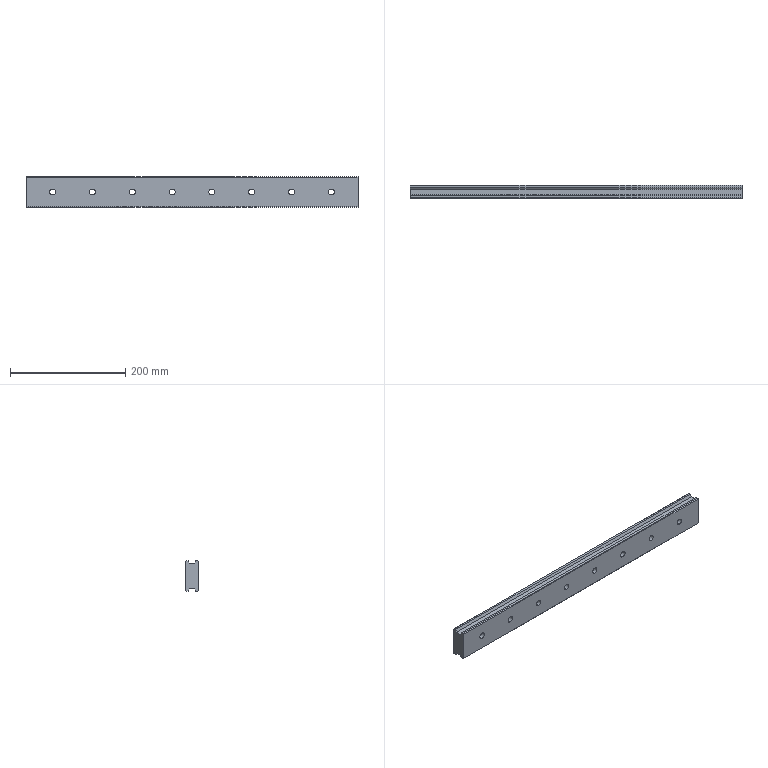Part | SolidWorks | features BaseBody 1 | 1 solid | 58 faces | box 576.923 x 23.077 x 53.538 mm | volume 590551 mm3 | cylinder 32 | plane 26 | commonest cylinder face diameters 10.385 x16 23.077 x16